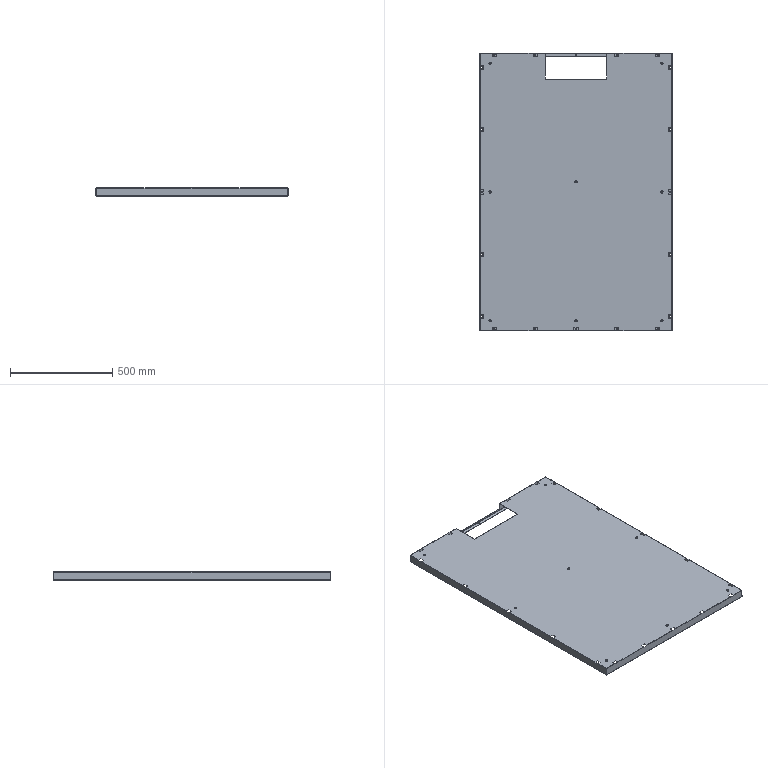Part | SolidWorks | features ICE 5, EdgeFlange 2, Cut 1, FlatPattern 1, SMBaseFlange 1, SheetMetal 1 | 1 solid | 376 faces | box 939 x 1359 x 40 mm | volume 1469027 mm3 | plane 238 | cylinder 122 | spline 16 | commonest cylinder face diameters 7 x50 0.4 x28 2.4 x28 11 x16